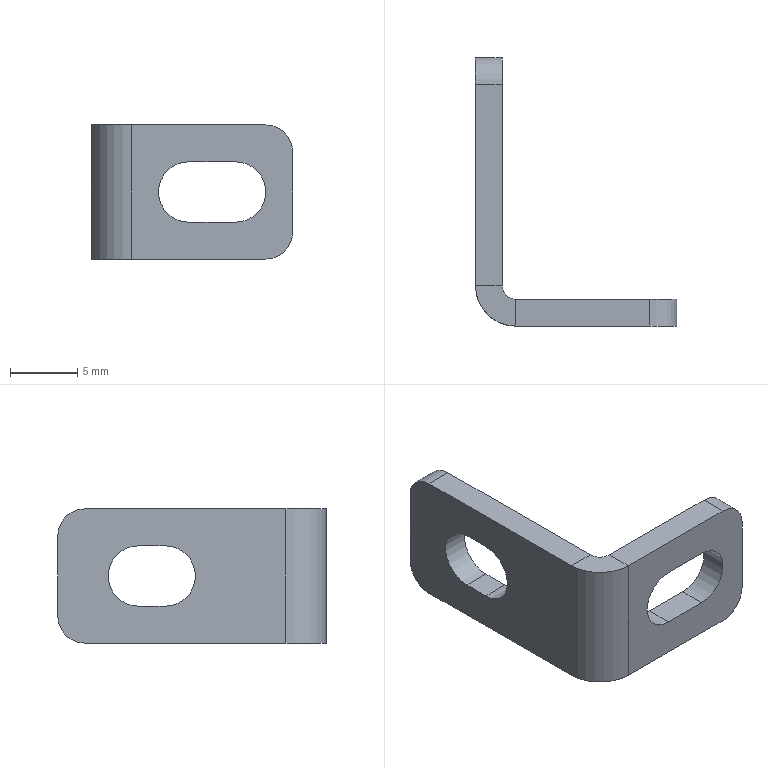Part | STEP file | power supply fixing sheet metal | 1 solid | 26 faces | box 15 x 20 x 10 mm | volume 522.847 mm3 | plane 16 | cylinder 10 | commonest cylinder face diameters 4 x4 4.5 x4 2 x1 6 x1